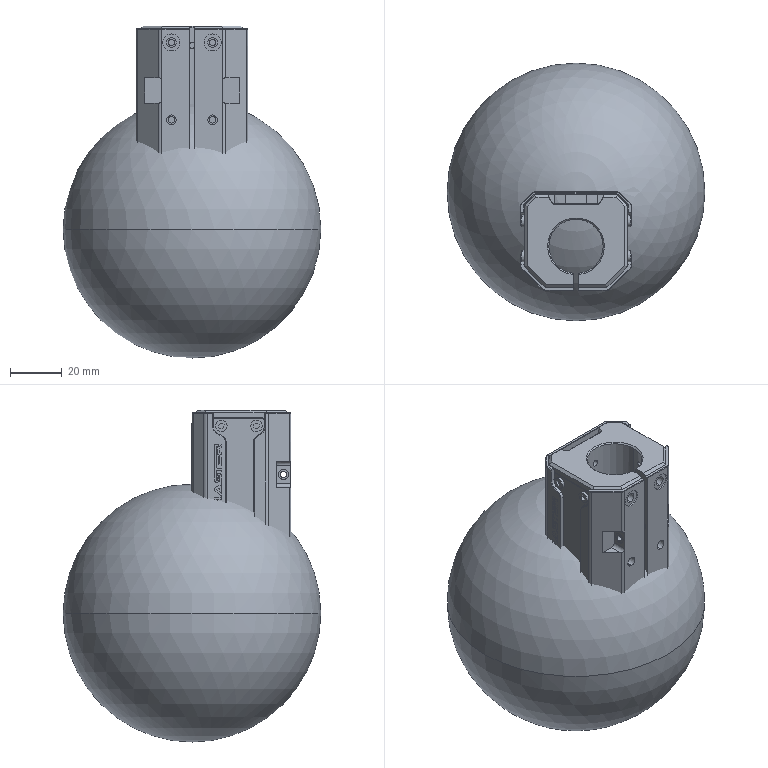Part | SolidWorks | 28 solids | 1345 faces | box 100 x 100 x 128.825 mm | volume 681485 mm3 | plane 702 | cylinder 447 | spline 128 | cone 64 | sphere 4 | commonest cylinder face diameters 3.8 x66 3.2 x55 4 x53 2 x50 2.5 x30 2.37 x22